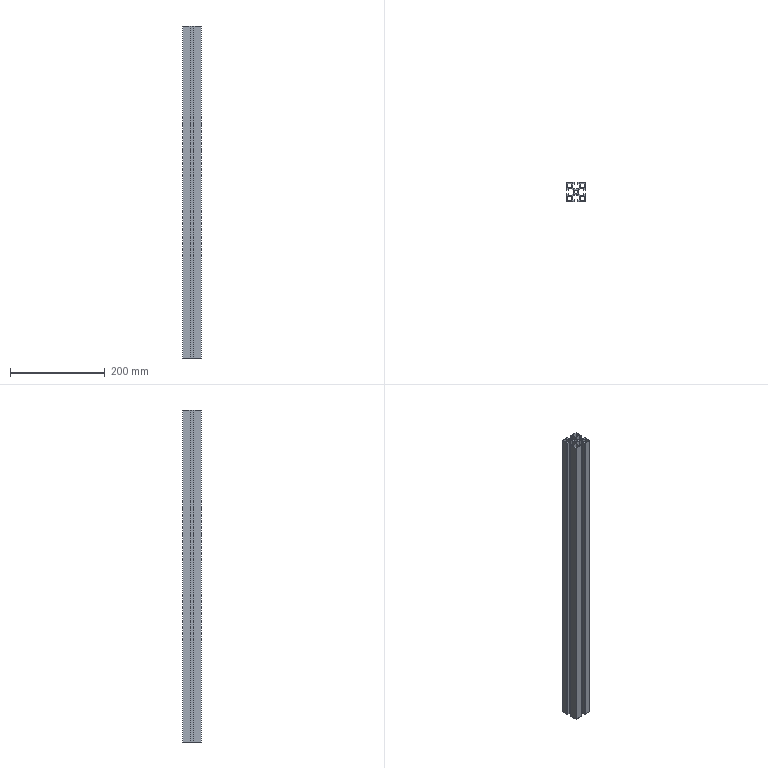Part | STEP file | 40_40_700_1-2 | 1 solid | 64 faces | box 40 x 40 x 700 mm | volume 367320 mm3 | plane 62 | cylinder 2 | commonest cylinder face diameters 6.8 x2